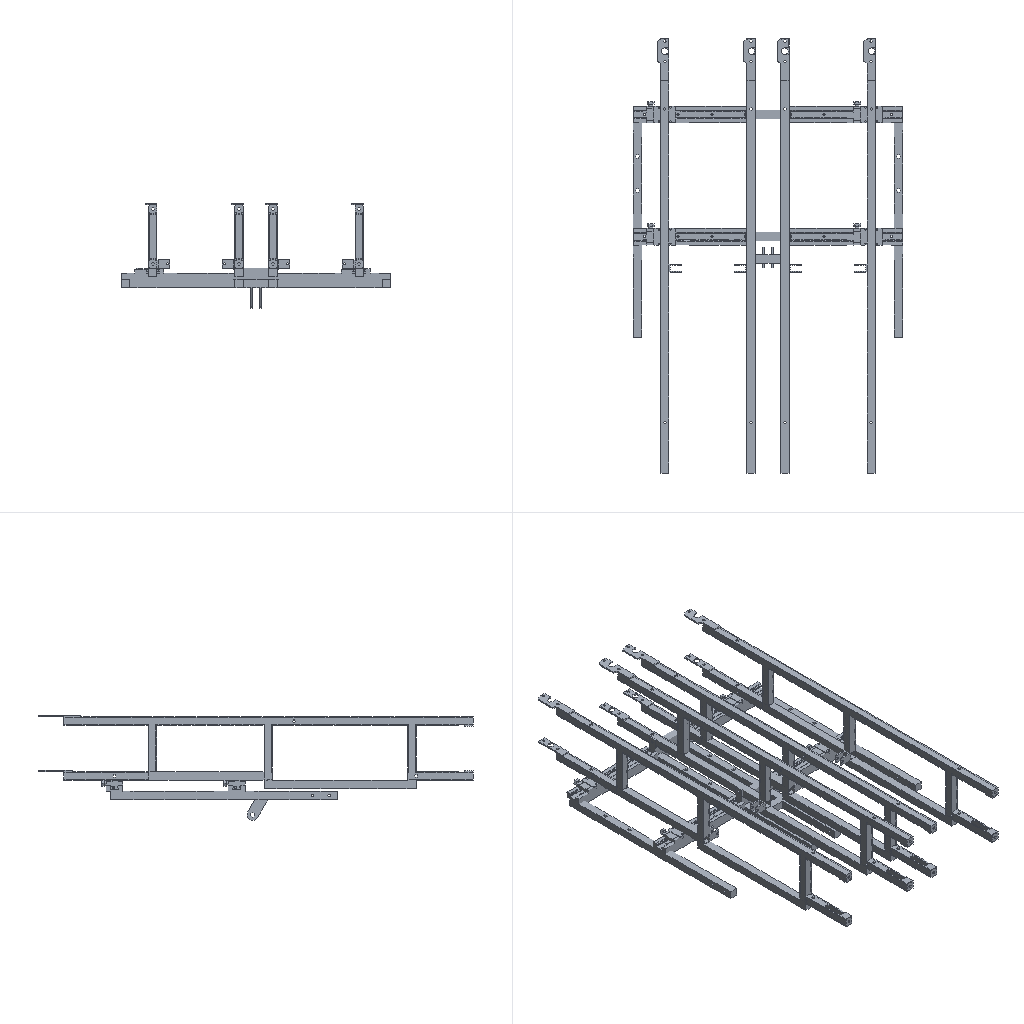Simulation study | ansys workbench
Set-up summary:
category,name,step,type,value,unit,region
solver,ansys_workbench
units,mm-N-s-tonne (MPa),,stated,"/units,MPA"
analysis,LS1,,modal,method=lanb; n_modes=6
load_step,LS1,LS1,modal
mesh,nodes,,,63940
mesh,elements,,,37557
element_type,SOLID187,,,27969
element_type,TARGE170,,,4616
element_type,CONTA174,,,4616
element_type,SOLID186,,,356
material,Structural Steel,,E,200000,tonne s^-2 mm^-1
material,Structural Steel,,nu,0.3
material,Structural Steel,,density,7.85e-09,tonne mm^-3
material,Structural Steel,,conductivity,60.5,tonne mm s^-3 C^-1
material,Structural Steel,,specific_heat,4.34e+08,mm^2 s^-2 C^-1
material,Structural Steel,,cte,1.2e-05,C^-1
material,Structural Steel,,permeability,10000
material,Structural Steel,,resistivity,0.00017,ohm mm
bc,Fixed Supports,model,fixed,[dofs=ALL],,_FIXEDSU
contact,Contact Region 3,,bonded (always),element=CONTA174
contact,Contact Region 4,,bonded (always),element=CONTA174
contact,Contact Region 7,,bonded (always),element=CONTA174
contact,Contact Region 8,,bonded (always),element=CONTA174
contact,Contact Region 9,,bonded (always),element=CONTA174
contact,Contact Region 10,,bonded (always),element=CONTA174
contact,Contact Region 11,,bonded (always),element=CONTA174
contact,Contact Region 12,,bonded (always),element=CONTA174
contact,Contact Region 13,,bonded (always),element=CONTA174
contact,Contact Region 14,,bonded (always),element=CONTA174
contact,Contact Region 15,,bonded (always),element=CONTA174
contact,Contact Region 16,,bonded (always),element=CONTA174
contact,Contact Region 17,,bonded (always),element=CONTA174
contact,Contact Region 18,,bonded (always),element=CONTA174
contact,Contact Region 19,,bonded (always),element=CONTA174
contact,Contact Region 20,,bonded (always),element=CONTA174
contact,Contact Region 21,,bonded (always),element=CONTA174
contact,Contact Region 22,,bonded (always),element=CONTA174
contact,Contact Region 23,,bonded (always),element=CONTA174
contact,Contact Region 24,,bonded (always),element=CONTA174
contact,Contact Region 25,,bonded (always),element=CONTA174
contact,Contact Region 26,,bonded (always),element=CONTA174
contact,Contact Region 27,,bonded (always),element=CONTA174
contact,Contact Region 28,,bonded (always),element=CONTA174
contact,Contact Region 29,,bonded (always),element=CONTA174
contact,Contact Region 30,,bonded (always),element=CONTA174
contact,Contact Region 31,,bonded (always),element=CONTA174
contact,Contact Region 32,,bonded (always),element=CONTA174
contact,Contact Region 33,,bonded (always),element=CONTA174
contact,Contact Region 34,,bonded (always),element=CONTA174
named_set,_FIXEDSU,,node,977
Ansys APDL input file, long lists of numbers shortened:
/batch
/config,noeldb,1     ! force off writing results to database
*get,_wallstrt,active,,time,wall
! ANSYS input file written by Workbench version 2022 R1
! File used for geometry attach:
/title,wbnew--__ (B5)
! ****** Begin Custom Load Command Snippet ******
/COM, ACT Extensions:
/COM,     LSDYNA, 2021.1
/COM,
! ****** End   Custom Load Command Snippet ******
*DIM,_wb_ProjectScratch_dir,string,248
_wb_ProjectScratch_dir(1) = ''
*DIM,_wb_SolverFiles_dir,string,248
_wb_SolverFiles_dir(1) = ''
*DIM,_wb_userfiles_dir,string,248
_wb_userfiles_dir(1) = ''
/com,--- Data in consistent NMM units. See Solving Units in the help system for more information.
/units,MPA
/nopr
/wb,file,start              !  signify a WB generated input file
/prep7
! Turn off shape checking because checks already performed inside WB mesher.
! See help system for more information.
SHPP,OFF,,NOWARN
/nolist
etcon,set             ! allow ANSYS to choose best KEYOP's for 180x elements, resets any applicable keyopt to MAPDL defaults
/com,*********** Nodes for the whole assembly ***********
nblock,3,,70334
(1i9,3e20.9e3)
    87706     2.735594585E+02    -1.426426848E+02     7.515063509E+01
! (63939 more lines like these left out)
-1
/wb,elem,start            !  set before creation of elements
/com,*********** Elements for Body 1 "_____|__-________|____-____1" ***********
et,1,187
eblock,19,solid,,304
(19i9)
        1        1        1        1        0        0        0        0       10        0        1    39130    39201    39135    39271    39293    39323    39291    39294
! (607 more lines like these left out)
-1
/com,*********** Elements for Body 2 "_____|__-________|____-____1[2]" ***********
et,2,187
eblock,19,solid,,304
(19i9)
        2        2        2        2        0        0        0        0       10        0      305    39864    39935    39869    40005    40027    40057    40025    40028
! (607 more lines like these left out)
-1
/com,*********** Elements for Body 3 "_____|__-________|____-____1[3]" ***********
et,3,187
eblock,19,solid,,304
(19i9)
        3        3        3        3        0        0        0        0       10        0      609    86974    87045    86979    87115    87137    87167    87135    87138
! (607 more lines like these left out)
-1
/com,*********** Elements for Body 4 "_____|__-________|____-____1[4]" ***********
et,4,187
eblock,19,solid,,304
(19i9)
        4        4        4        4        0        0        0        0       10        0      913    87708    87779    87713    87849    87871    87901    87869    87872
! (607 more lines like these left out)
-1
/com,*********** Elements for Body 5 "__-____|____-____10" ***********
et,5,187
eblock,19,solid,,2953
(19i9)
        5        5        5        5        0        0        0        0       10        0     1217    89493    89674    89630    89636    94828    95050    94825    94827
! (5905 more lines like these left out)
-1
! (24 more sections like these left out)
/wb,elem,end               !  done creating elements
/com,*********** Send User Defined Coordinate System(s) ***********
csys,0
toffst,273.15,  ! Temperature offset from absolute zero
/com,*********** Set Reference Temperature ***********
tref,22.
/wb,mat,start              !  starting to send materials
/com,*********** Send Materials ***********
Temperature = 'TEMP' ! Temperature
MP,DENS,1,7.85e-09,	! tonne mm^-3
MP,ALPX,1,1.2e-05,	! C^-1
MP,C,1,434000000,	! mm^2 s^-2 C^-1
MP,KXX,1,60.5,	! tonne mm s^-3 C^-1
MP,RSVX,1,0.00017,	! ohm mm
MP,EX,1,200000,	! tonne s^-2 mm^-1
MP,NUXY,1,0.3,
MP,MURX,1,10000,
Temperature = 'TEMP' ! Temperature
MP,DENS,2,7.85e-09,	! tonne mm^-3
MP,ALPX,2,1.2e-05,	! C^-1
MP,C,2,434000000,	! mm^2 s^-2 C^-1
MP,KXX,2,60.5,	! tonne mm s^-3 C^-1
MP,RSVX,2,0.00017,	! ohm mm
MP,EX,2,200000,	! tonne s^-2 mm^-1
MP,NUXY,2,0.3,
MP,MURX,2,10000,
Temperature = 'TEMP' ! Temperature
MP,DENS,3,7.85e-09,	! tonne mm^-3
MP,ALPX,3,1.2e-05,	! C^-1
MP,C,3,434000000,	! mm^2 s^-2 C^-1
MP,KXX,3,60.5,	! tonne mm s^-3 C^-1
MP,RSVX,3,0.00017,	! ohm mm
MP,EX,3,200000,	! tonne s^-2 mm^-1
MP,NUXY,3,0.3,
MP,MURX,3,10000,
Temperature = 'TEMP' ! Temperature
MP,DENS,4,7.85e-09,	! tonne mm^-3
MP,ALPX,4,1.2e-05,	! C^-1
MP,C,4,434000000,	! mm^2 s^-2 C^-1
MP,KXX,4,60.5,	! tonne mm s^-3 C^-1
MP,RSVX,4,0.00017,	! ohm mm
MP,EX,4,200000,	! tonne s^-2 mm^-1
MP,NUXY,4,0.3,
MP,MURX,4,10000,
Temperature = 'TEMP' ! Temperature
MP,DENS,5,7.85e-09,	! tonne mm^-3
MP,ALPX,5,1.2e-05,	! C^-1
MP,C,5,434000000,	! mm^2 s^-2 C^-1
MP,KXX,5,60.5,	! tonne mm s^-3 C^-1
MP,RSVX,5,0.00017,	! ohm mm
MP,EX,5,200000,	! tonne s^-2 mm^-1
MP,NUXY,5,0.3,
MP,MURX,5,10000,
Temperature = 'TEMP' ! Temperature
MP,DENS,6,7.85e-09,	! tonne mm^-3
MP,ALPX,6,1.2e-05,	! C^-1
MP,C,6,434000000,	! mm^2 s^-2 C^-1
MP,KXX,6,60.5,	! tonne mm s^-3 C^-1
MP,RSVX,6,0.00017,	! ohm mm
MP,EX,6,200000,	! tonne s^-2 mm^-1
MP,NUXY,6,0.3,
MP,MURX,6,10000,
Temperature = 'TEMP' ! Temperature
MP,DENS,7,7.85e-09,	! tonne mm^-3
MP,ALPX,7,1.2e-05,	! C^-1
MP,C,7,434000000,	! mm^2 s^-2 C^-1
MP,KXX,7,60.5,	! tonne mm s^-3 C^-1
MP,RSVX,7,0.00017,	! ohm mm
MP,EX,7,200000,	! tonne s^-2 mm^-1
MP,NUXY,7,0.3,
MP,MURX,7,10000,
Temperature = 'TEMP' ! Temperature
MP,DENS,8,7.85e-09,	! tonne mm^-3
MP,ALPX,8,1.2e-05,	! C^-1
MP,C,8,434000000,	! mm^2 s^-2 C^-1
MP,KXX,8,60.5,	! tonne mm s^-3 C^-1
MP,RSVX,8,0.00017,	! ohm mm
MP,EX,8,200000,	! tonne s^-2 mm^-1
MP,NUXY,8,0.3,
MP,MURX,8,10000,
Temperature = 'TEMP' ! Temperature
MP,DENS,9,7.85e-09,	! tonne mm^-3
MP,ALPX,9,1.2e-05,	! C^-1
MP,C,9,434000000,	! mm^2 s^-2 C^-1
MP,KXX,9,60.5,	! tonne mm s^-3 C^-1
MP,RSVX,9,0.00017,	! ohm mm
MP,EX,9,200000,	! tonne s^-2 mm^-1
! (182 more lines like these left out)
/wb,mat,end                !  done sending materials
!************************* Model Summary ********************
!_____|__-________|____-____1,	结构钢,	matid,	1
!_____|__-________|____-____1[2],	结构钢,	matid,	2
!_____|__-________|____-____1[3],	结构钢,	matid,	3
! (28 more lines like these left out)
*get,_xmin,node,,mnloc,x
*get,_ymin,node,,mnloc,y
*get,_zmin,node,,mnloc,z
*get,_xmax,node,,mxloc,x
*get,_ymax,node,,mxloc,y
*get,_zmax,node,,mxloc,z
_ASMDIAG=(_xmax-_xmin)*(_xmax-_xmin)+(_ymax-_ymin)*(_ymax-_ymin)+(_zmax-_zmin)*(_zmax-_zmin)
_ASMDIAG=SQRT(_ASMDIAG)
/wb,contact,start          !  starting to send contact
/com,*********** Create Contact "接触区域 3" ***********
/com,            Real Constant Set For Above Contact Is 31 & 30
*set,tid,31
*set,cid,30
r,tid
r,cid
et,tid,170
et,cid,174
eblock,10,,,16
(15i9)
   116709       31       31       31        0    39224    39264    39225    39225    39740    39743    39225    39736
! (15 more lines like these left out)
-1
eblock,10,,,16
(15i9)
   116725       30       30       30        0    39224    39264    39225    39225    39740    39743    39225    39736
! (15 more lines like these left out)
-1
eblock,10,,,10
(15i9)
   116741       30       31       30        0   121146   121173   121641   121641   123910   124098   121641   123913
! (9 more lines like these left out)
-1
eblock,10,,,10
(15i9)
   116751       31       30       31        0   121146   121173   121641   121641   123910   124098   121641   123913
! (9 more lines like these left out)
-1
keyo,cid,8,2               ! auto create asymmetric contact (from Program Controlled setting)
keyo,cid,10,0              ! adjust contact stiffness each NR iteration (from Program Controlled setting)
keyo,cid,12,5              ! bonded always
keyo,cid,18,1              ! small sliding turned on by application
keyo,cid,2,0               ! augmented Lagrange (from Program Controlled setting)
keyo,cid,4,0               ! on Gauss point (from Program Controlled setting)
keyo,cid,9,1               ! ignore initial gaps/penetration
keyo,cid,7,0               ! No Prediction
rmod,tid,3,10.      ! FKN
rmod,tid,5,0.       ! ICONT
rmod,tid,6,0.       ! PINB
rmod,tid,10,0.      ! CNOF
rmod,tid,12,0.      ! FKT
rmod,tid,36,122     ! WB DSID
rmod,cid,3,10.      ! FKN
rmod,cid,5,0.       ! ICONT
rmod,cid,6,0.       ! PINB
rmod,cid,10,0.      ! CNOF
rmod,cid,12,0.      ! FKT
rmod,cid,36,122     ! WB DSID
/com,*********** Create Contact "接触区域 4" ***********
/com,            Real Constant Set For Above Contact Is 33 & 32
*set,tid,33
*set,cid,32
r,tid
r,cid
et,tid,170
et,cid,174
eblock,10,,,16
(15i9)
   116761       33       33       33        0    39958    39998    39959    39959    40474    40477    39959    40470
! (15 more lines like these left out)
-1
eblock,10,,,16
(15i9)
   116777       32       32       32        0    39958    39998    39959    39959    40474    40477    39959    40470
! (15 more lines like these left out)
-1
eblock,10,,,10
(15i9)
   116793       32       33       32        0   128606   129084   129079   129079   131992   134170   129079   131990
! (9 more lines like these left out)
-1
eblock,10,,,10
(15i9)
   116803       33       32       33        0   128606   129084   129079   129079   131992   134170   129079   131990
! (9 more lines like these left out)
-1
keyo,cid,8,2               ! auto create asymmetric contact (from Program Controlled setting)
keyo,cid,10,0              ! adjust contact stiffness each NR iteration (from Program Controlled setting)
keyo,cid,12,5              ! bonded always
keyo,cid,18,1              ! small sliding turned on by application
keyo,cid,2,0               ! augmented Lagrange (from Program Controlled setting)
keyo,cid,4,0               ! on Gauss point (from Program Controlled setting)
keyo,cid,9,1               ! ignore initial gaps/penetration
keyo,cid,7,0               ! No Prediction
rmod,tid,3,10.      ! FKN
rmod,tid,5,0.       ! ICONT
rmod,tid,6,0.       ! PINB
rmod,tid,10,0.      ! CNOF
rmod,tid,12,0.      ! FKT
rmod,tid,36,125     ! WB DSID
rmod,cid,3,10.      ! FKN
rmod,cid,5,0.       ! ICONT
rmod,cid,6,0.       ! PINB
rmod,cid,10,0.      ! CNOF
rmod,cid,12,0.      ! FKT
rmod,cid,36,125     ! WB DSID
/com,*********** Create Contact "接触区域 7" ***********
/com,            Real Constant Set For Above Contact Is 35 & 34
*set,tid,35
*set,cid,34
r,tid
r,cid
et,tid,170
et,cid,174
eblock,10,,,16
(15i9)
   116813       35       35       35        0    87068    87108    87069    87069    87584    87587    87069    87580
! (15 more lines like these left out)
-1
eblock,10,,,16
(15i9)
   116829       34       34       34        0    87068    87108    87069    87069    87584    87587    87069    87580
! (15 more lines like these left out)
-1
eblock,10,,,10
(15i9)
   116845       34       35       34        0   135973   136451   136446   136446   139359   141537   136446   139357
! (9 more lines like these left out)
-1
eblock,10,,,10
(15i9)
   116855       35       34       35        0   135973   136451   136446   136446   139359   141537   136446   139357
! (9 more lines like these left out)
-1
keyo,cid,8,2               ! auto create asymmetric contact (from Program Controlled setting)
keyo,cid,10,0              ! adjust contact stiffness each NR iteration (from Program Controlled setting)
keyo,cid,12,5              ! bonded always
keyo,cid,18,1              ! small sliding turned on by application
keyo,cid,2,0               ! augmented Lagrange (from Program Controlled setting)
keyo,cid,4,0               ! on Gauss point (from Program Controlled setting)
keyo,cid,9,1               ! ignore initial gaps/penetration
keyo,cid,7,0               ! No Prediction
rmod,tid,3,10.      ! FKN
rmod,tid,5,0.       ! ICONT
rmod,tid,6,0.       ! PINB
rmod,tid,10,0.      ! CNOF
rmod,tid,12,0.      ! FKT
rmod,tid,36,134     ! WB DSID
rmod,cid,3,10.      ! FKN
rmod,cid,5,0.       ! ICONT
rmod,cid,6,0.       ! PINB
rmod,cid,10,0.      ! CNOF
rmod,cid,12,0.      ! FKT
rmod,cid,36,134     ! WB DSID
/com,*********** Create Contact "接触区域 8" ***********
/com,            Real Constant Set For Above Contact Is 37 & 36
*set,tid,37
*set,cid,36
r,tid
r,cid
et,tid,170
et,cid,174
eblock,10,,,16
(15i9)
   116865       37       37       37        0    87802    87842    87803    87803    88318    88321    87803    88314
! (15 more lines like these left out)
-1
eblock,10,,,16
(15i9)
   116881       36       36       36        0    87802    87842    87803    87803    88318    88321    87803    88314
! (15 more lines like these left out)
-1
eblock,10,,,10
(15i9)
   116897       36       37       36        0   143247   143274   143742   143742   146011   146199   143742   146014
! (9 more lines like these left out)
-1
eblock,10,,,10
(15i9)
   116907       37       36       37        0   143247   143274   143742   143742   146011   146199   143742   146014
! (9 more lines like these left out)
-1
keyo,cid,8,2               ! auto create asymmetric contact (from Program Controlled setting)
keyo,cid,10,0              ! adjust contact stiffness each NR iteration (from Program Controlled setting)
keyo,cid,12,5              ! bonded always
keyo,cid,18,1              ! small sliding turned on by application
keyo,cid,2,0               ! augmented Lagrange (from Program Controlled setting)
keyo,cid,4,0               ! on Gauss point (from Program Controlled setting)
keyo,cid,9,1               ! ignore initial gaps/penetration
keyo,cid,7,0               ! No Prediction
rmod,tid,3,10.      ! FKN
rmod,tid,5,0.       ! ICONT
rmod,tid,6,0.       ! PINB
rmod,tid,10,0.      ! CNOF
rmod,tid,12,0.      ! FKT
rmod,tid,36,137     ! WB DSID
rmod,cid,3,10.      ! FKN
rmod,cid,5,0.       ! ICONT
rmod,cid,6,0.       ! PINB
rmod,cid,10,0.      ! CNOF
rmod,cid,12,0.      ! FKT
rmod,cid,36,137     ! WB DSID
/com,*********** Create Contact "接触区域 9" ***********
/com,            Real Constant Set For Above Contact Is 39 & 38
*set,tid,39
*set,cid,38
r,tid
r,cid
et,tid,170
et,cid,174
eblock,10,,,38
(15i9)
   116917       39       39       39        0    88986    88991    88992    88992    92920    92941    88992    92921
! (37 more lines like these left out)
-1
eblock,10,,,38
(15i9)
   116955       38       38       38        0    88986    88991    88992    88992    92920    92941    88992    92921
! (37 more lines like these left out)
-1
eblock,10,,,104
(15i9)
   116993       38       39       38        0    95267    95278    95277    95277    96768    96851    95277    96767
! (103 more lines like these left out)
-1
eblock,10,,,104
(15i9)
   117097       39       38       39        0    95267    95278    95277    95277    96768    96851    95277    96767
! (103 more lines like these left out)
-1
keyo,cid,8,2               ! auto create asymmetric contact (from Program Controlled setting)
keyo,cid,10,0              ! adjust contact stiffness each NR iteration (from Program Controlled setting)
keyo,cid,12,5              ! bonded always
keyo,cid,18,1              ! small sliding turned on by application
keyo,cid,2,0               ! augmented Lagrange (from Program Controlled setting)
keyo,cid,4,0               ! on Gauss point (from Program Controlled setting)
keyo,cid,9,1               ! ignore initial gaps/penetration
keyo,cid,7,0               ! No Prediction
rmod,tid,3,10.      ! FKN
rmod,tid,5,0.       ! ICONT
rmod,tid,6,0.       ! PINB
rmod,tid,10,0.      ! CNOF
rmod,tid,12,0.      ! FKT
rmod,tid,36,140     ! WB DSID
rmod,cid,3,10.      ! FKN
rmod,cid,5,0.       ! ICONT
rmod,cid,6,0.       ! PINB
rmod,cid,10,0.      ! CNOF
rmod,cid,12,0.      ! FKT
rmod,cid,36,140     ! WB DSID
! (25 more sections like these left out)
/wb,contact,end            !  done creating contacts
/golist
/wb,load,start             !  starting to send loads
/com,*********** Fixed Supports ***********
CMBLOCK,_FIXEDSU,NODE,      977
(8i10)
     88492     88493     88494     88495     88500     88501     88502     88503
! (122 more lines like these left out)
cmsel,s,_FIXEDSU
d,all,all
nsel,all
/gst,on,on
fini
*get,_numnode,node,0,count
*get,_numelem,elem,0,count
*get, _MAXELEMNUM, elem, 0, NUM, MAX
*get, _MAXNODENUM, node, 0, NUM, MAX
*get, _MAXELEMTYPE, etyp, 0, NUM, MAX
*get, _MAXREALCONST, real, 0, NUM, MAX
/go
/wb,load,end               !  done creating loads
/com,--- Number of total nodes = %_numnode%
/com,--- Number of contact elements = 9232
/com,--- Number of spring elements = 0
/com,--- Number of bearing elements = 0
/com,--- Number of solid elements = 28325
/com,--- Number of condensed parts = 0
/com,--- Number of total elements = %_numelem%
*get,_wallbsol,active,,time,wall
/solu
antype,2                   ! modal analysis
_thickRatio=  0     ! Ratio of thick parts in the model
modopt,lanb,6
outres,erase
outres,all,none
outres,nsol,all
outres,etmp,all
mxpand                    ! default expand in case of complex solution
dmpopt,esav,no
dmpopt,emat,no
dmpopt,full,no
! *********** WB SOLVE COMMAND ***********
! check interactive state
*get,ANSINTER_,active,,int
*if,ANSINTER_,ne,0,then
/eof
*endif
solve
/com *************** Write FE CONNECTORS *********
CEWRITE,file,ce,,INTE
*get,_nmodalsolproc,active,0,numcpu
fini
/nopr
*get,_numnode,node,0,count
*get,_numelem,elem,0,count
*get, _MAXELEMNUM, elem, 0, NUM, MAX
*get, _MAXNODENUM, node, 0, NUM, MAX,,,INTERNAL
*get, _MAXELEMTYPE, etyp, 0, NUM, MAX
*get, _MAXREALCONST, real, 0, NUM, MAX
/gopr
*get,_wallasol,active,,time,wall
/post1
/nopr
*dim,_direction,CHAR,6,1
_direction(1) = 'X'
_direction(2) = 'Y'
_direction(3) = 'Z'
_direction(4) = 'ROTX'
_direction(5) = 'ROTY'
_direction(6) = 'ROTZ'
*get,_lastLS,active,0,set,LSTP
*get,_beginset,active,0,set,nset,first,_lastLS
*get,_endset,active,0,set,nset,last,_lastLS
_nummodes = 0
*if,_endset,gt,0,then
_nummodes = _endset - _beginset + 1
*endif
*do,i_mode,1,_nummodes
   *do,j_component,1,6
			*get,PFACT_%i_mode%_%j_component%,MODE,%i_mode%,PFACT,,DIREC,_direction(%j_component%)
   *enddo
*enddo
*dim,_tmdirection,CHAR,6,1
_tmdirection(1) = 'X'
_tmdirection(2) = 'Y'
_tmdirection(3) = 'Z'
_tmdirection(4) = 'X'
_tmdirection(5) = 'Y'
_tmdirection(6) = 'Z'
*do,j_component,1,6
    *if,j_component,gt,3,then
        *get,TOTALMASS_%j_component%,ELEM,0,IOR,_tmdirection(%j_component%)
    *else
        *get,TOTALMASS_%j_component%,ELEM,0,MTOT,_tmdirection(%j_component%)
    *endif
*enddo
/gopr
xmlo,ENCODING,ISO-8859-1
xmlo,parm
/xml,parm,xml
fini
/gopr
*get,_walldone,active,,time,wall
_preptime=(_wallbsol-_wallstrt)*3600
_solvtime=(_wallasol-_wallbsol)*3600
_posttime=(_walldone-_wallasol)*3600
_totaltim=(_walldone-_wallstrt)*3600
*get,_dlbratio,active,0,solu,dlbr
*get,_combtime,active,0,solu,comb
*get,_ssmode,active,0,solu,ssmm
*get,_ndofs,active,0,solu,ndof
/fclean				!clean distributed files
/com,--- Total number of nodes = %_numnode%
/com,--- Total number of elements = %_numelem%
/com,--- Element load balance ratio = %_dlbratio%
/com,--- Time to combine distributed files = %_combtime%
/com,--- Sparse memory mode = %_ssmode%
/com,--- Number of DOF = %_ndofs%
/wb,file,end               ! done with WB generated input
Results summary:
result,analyses[0].index,,,1
result,analyses[0].system,,,SYS
result,analyses[0].deck,,,deck.dat
result,analyses[0].solve_status,,,completed
result,analyses[0].analysis_type,,,modal
result,analyses[0].physics,,,mechanical
result,analyses[0].unit_system,,,"NMM: mm, ton, N, s, mV, mA, degC"
result,analyses[0].n_sets,,,6
result,analyses[0].modal_frequencies_hz[1],,,13.485
result,analyses[0].modal_frequencies_hz[2],,,13.488
result,analyses[0].modal_frequencies_hz[3],,,15.488
result,analyses[0].modal_frequencies_hz[4],,,15.5
result,analyses[0].modal_frequencies_hz[5],,,38.396
result,analyses[0].modal_frequencies_hz[6],,,38.601